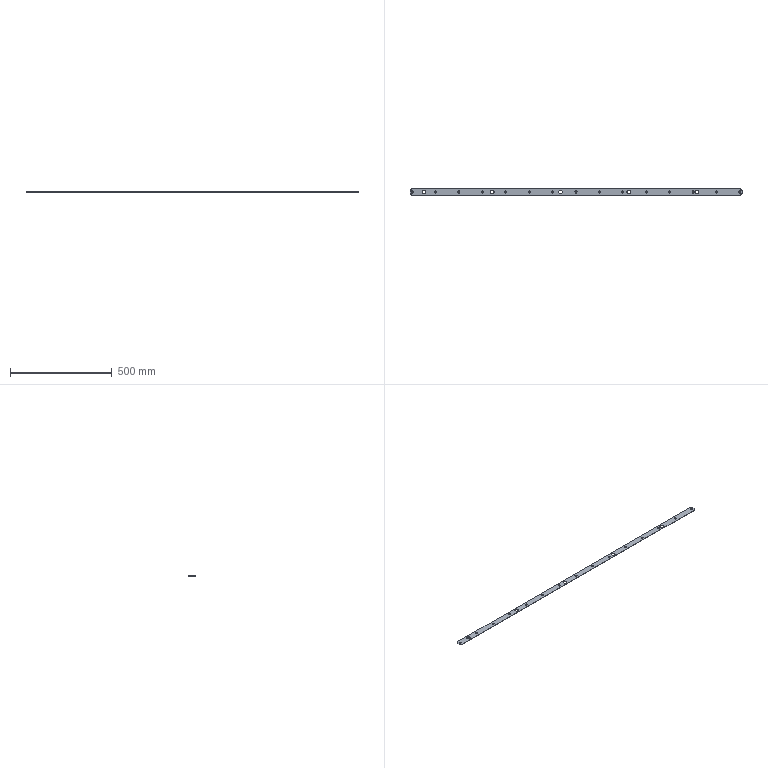Part | SolidWorks | features Fillet 1, FlatPattern 1, SMBaseFlange 1, SheetMetal 1 | 1 solid | 50 faces | box 1630 x 30 x 1.6 mm | volume 74182 mm3 | cylinder 44 | plane 6 | commonest cylinder face diameters 10 x30 18 x10 20 x4